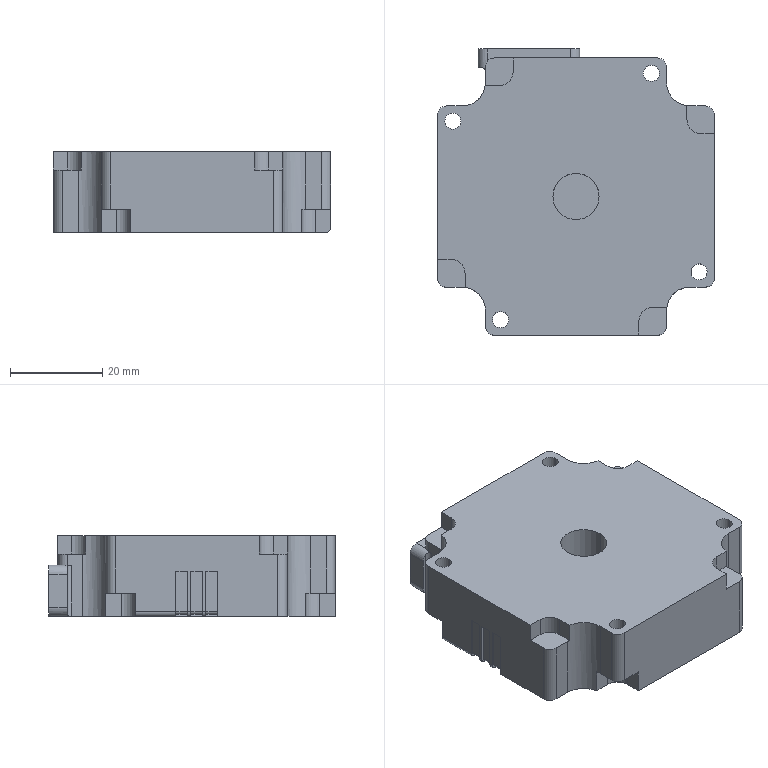Part | STEP file | 31100246--1-SOLI00_1_1_1 | 1 solid | 127 faces | box 60 x 62 x 17.5 mm | volume 52728 mm3 | plane 75 | cylinder 50 | spline 2 | commonest cylinder face diameters 4 x13 2 x11 3.5 x8 6 x8 10 x6 1 x4